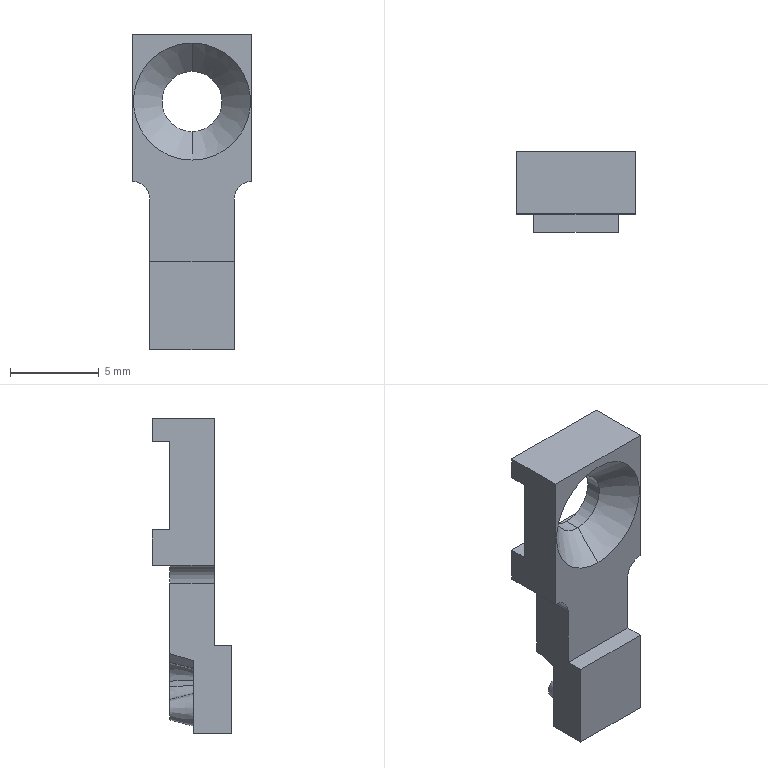Part | SolidWorks | features Cut 6, Chamfer 2, ICE 2, Extrusion 1, Fillet 1, HoleWzd 1 | 1 solid | 35 faces | box 6.75 x 4.5 x 17.8 mm | volume 246.564 mm3 | plane 23 | cone 8 | cylinder 4 | commonest cylinder face diameters 2 x2 3.4 x2
STEP:
#1=CARTESIAN_POINT('',(0.,-1.9,7.15));
#2=VERTEX_POINT('',#1);
#3=CARTESIAN_POINT('',(0.,-1.9,3.75));
#4=VERTEX_POINT('',#3);
#5=CARTESIAN_POINT('',(0.,-1.9,5.45));
#6=DIRECTION('',(0.,-1.,0.));
#7=DIRECTION('',(0.,0.,-1.));
#8=AXIS2_PLACEMENT_3D('',#5,#6,#7);
#9=CIRCLE('',#8,1.7);
#10=EDGE_CURVE('',#2,#4,#9,.T.);
#11=ORIENTED_EDGE('',*,*,#10,.F.);
#12=CARTESIAN_POINT('',(0.,-3.5,8.75));
#13=VERTEX_POINT('',#12);
#14=CARTESIAN_POINT('',(0.,-3.5,8.75));
#15=DIRECTION('',(0.,-0.7071,0.7071));
#16=VECTOR('',#15,1000.);
#17=LINE('',#14,#16);
#18=EDGE_CURVE('',#2,#13,#17,.T.);
#19=ORIENTED_EDGE('',*,*,#18,.T.);
#20=CARTESIAN_POINT('',(0.,-3.5,2.15));
#21=VERTEX_POINT('',#20);
#22=CARTESIAN_POINT('',(0.,-3.5,5.45));
#23=DIRECTION('',(0.,-1.,0.));
#24=DIRECTION('',(0.,0.,-1.));
#25=AXIS2_PLACEMENT_3D('',#22,#23,#24);
#26=CIRCLE('',#25,3.3);
#27=EDGE_CURVE('',#13,#21,#26,.T.);
#28=ORIENTED_EDGE('',*,*,#27,.T.);
#29=CARTESIAN_POINT('',(0.,-3.5,2.15));
#30=DIRECTION('',(0.,-0.7071,-0.7071));
#31=VECTOR('',#30,1000.);
#32=LINE('',#29,#31);
#33=EDGE_CURVE('',#4,#21,#32,.T.);
#34=ORIENTED_EDGE('',*,*,#33,.F.);
#35=EDGE_LOOP('',(#11,#19,#28,#34));
#36=FACE_OUTER_BOUND('',#35,.T.);
#37=CARTESIAN_POINT('',(0.,-3.5,5.45));
#38=DIRECTION('',(0.,-1.,0.));
#39=DIRECTION('',(0.,0.,-1.));
#40=AXIS2_PLACEMENT_3D('',#37,#38,#39);
#41=CONICAL_SURFACE('',#40,3.3,0.7854);
#42=ADVANCED_FACE('',(#36),#41,.F.);
#43=CARTESIAN_POINT('',(0.,-1.,7.15));
#44=VERTEX_POINT('',#43);
#45=CARTESIAN_POINT('',(0.,-1.,3.75));
#46=VERTEX_POINT('',#45);
#47=CARTESIAN_POINT('',(0.,-1.,5.45));
#48=DIRECTION('',(0.,-1.,0.));
#49=DIRECTION('',(0.,0.,-1.));
#50=AXIS2_PLACEMENT_3D('',#47,#48,#49);
#51=CIRCLE('',#50,1.7);
#52=EDGE_CURVE('',#44,#46,#51,.T.);
#53=ORIENTED_EDGE('',*,*,#52,.F.);
#54=CARTESIAN_POINT('',(0.,-3.5,7.15));
#55=DIRECTION('',(0.,-1.,0.));
#56=VECTOR('',#55,1000.);
#57=LINE('',#54,#56);
#58=EDGE_CURVE('',#44,#2,#57,.T.);
#59=ORIENTED_EDGE('',*,*,#58,.T.);
#60=ORIENTED_EDGE('',*,*,#10,.T.);
#61=CARTESIAN_POINT('',(0.,-3.5,3.75));
#62=DIRECTION('',(0.,-1.,0.));
#63=VECTOR('',#62,1000.);
#64=LINE('',#61,#63);
#65=EDGE_CURVE('',#46,#4,#64,.T.);
#66=ORIENTED_EDGE('',*,*,#65,.F.);
#67=EDGE_LOOP('',(#53,#59,#60,#66));
#68=FACE_OUTER_BOUND('',#67,.T.);
#69=CARTESIAN_POINT('',(0.,-3.5,5.45));
#70=DIRECTION('',(0.,-1.,0.));
#71=DIRECTION('',(0.,0.,-1.));
#72=AXIS2_PLACEMENT_3D('',#69,#70,#71);
#73=CYLINDRICAL_SURFACE('',#72,1.7);
#74=ADVANCED_FACE('',(#68),#73,.F.);
#75=CARTESIAN_POINT('',(-1.503,-1.,-4.523));
#76=VERTEX_POINT('',#75);
#77=CARTESIAN_POINT('',(-1.512,-1.,-4.52));
#78=VERTEX_POINT('',#77);
#79=CARTESIAN_POINT('',(-1.503,-1.,-4.505));
#80=DIRECTION('',(0.,1.,0.));
#81=DIRECTION('',(0.,0.,-1.));
#82=AXIS2_PLACEMENT_3D('',#79,#80,#81);
#83=CIRCLE('',#82,0.01769);
#84=EDGE_CURVE('',#76,#78,#83,.T.);
#85=ORIENTED_EDGE('',*,*,#84,.T.);
#86=CARTESIAN_POINT('',(-2.375,-1.,-4.022));
#87=VERTEX_POINT('',#86);
#88=CARTESIAN_POINT('',(-5.278,-1.,-2.346));
#89=DIRECTION('',(-0.866,0.,0.5));
#90=VECTOR('',#89,1000.);
#91=LINE('',#88,#90);
#92=EDGE_CURVE('',#78,#87,#91,.T.);
#93=ORIENTED_EDGE('',*,*,#92,.T.);
#94=CARTESIAN_POINT('',(-2.375,-1.,-0.05));
#95=VERTEX_POINT('',#94);
#96=CARTESIAN_POINT('',(-2.375,-1.,-0.05));
#97=DIRECTION('',(0.,0.,1.));
#98=VECTOR('',#97,1000.);
#99=LINE('',#96,#98);
#100=EDGE_CURVE('',#87,#95,#99,.T.);
#101=ORIENTED_EDGE('',*,*,#100,.T.);
#102=CARTESIAN_POINT('',(-3.375,-1.,0.95));
#103=VERTEX_POINT('',#102);
#104=CARTESIAN_POINT('',(-3.375,-1.,-0.05));
#105=DIRECTION('',(0.,-1.,0.));
#106=DIRECTION('',(0.,0.,-1.));
#107=AXIS2_PLACEMENT_3D('',#104,#105,#106);
#108=CIRCLE('',#107,1.);
#109=EDGE_CURVE('',#95,#103,#108,.T.);
#110=ORIENTED_EDGE('',*,*,#109,.T.);
#111=CARTESIAN_POINT('',(3.375,-1.,0.95));
#112=VERTEX_POINT('',#111);
#113=CARTESIAN_POINT('',(-3.375,-1.,0.95));
#114=DIRECTION('',(1.,0.,0.));
#115=VECTOR('',#114,1000.);
#116=LINE('',#113,#115);
#117=EDGE_CURVE('',#103,#112,#116,.T.);
#118=ORIENTED_EDGE('',*,*,#117,.T.);
#119=CARTESIAN_POINT('',(2.375,-1.,-0.05));
#120=VERTEX_POINT('',#119);
#121=CARTESIAN_POINT('',(3.375,-1.,-0.05));
#122=DIRECTION('',(0.,-1.,0.));
#123=DIRECTION('',(0.,0.,-1.));
#124=AXIS2_PLACEMENT_3D('',#121,#122,#123);
#125=CIRCLE('',#124,1.);
#126=EDGE_CURVE('',#112,#120,#125,.T.);
#127=ORIENTED_EDGE('',*,*,#126,.T.);
#128=CARTESIAN_POINT('',(2.375,-1.,-7.053));
#129=VERTEX_POINT('',#128);
#130=CARTESIAN_POINT('',(2.375,-1.,-0.05));
#131=DIRECTION('',(0.,0.,-1.));
#132=VECTOR('',#131,1000.);
#133=LINE('',#130,#132);
#134=EDGE_CURVE('',#120,#129,#133,.T.);
#135=ORIENTED_EDGE('',*,*,#134,.T.);
#136=CARTESIAN_POINT('',(2.276,-1.,-7.225));
#137=VERTEX_POINT('',#136);
#138=CARTESIAN_POINT('',(4.403,-1.,-3.54));
#139=DIRECTION('',(-0.5,0.,-0.866));
#140=VECTOR('',#139,1000.);
#141=LINE('',#138,#140);
#142=EDGE_CURVE('',#129,#137,#141,.T.);
#143=ORIENTED_EDGE('',*,*,#142,.T.);
#144=CARTESIAN_POINT('',(0.8678,-1.,-7.225));
#145=VERTEX_POINT('',#144);
#146=CARTESIAN_POINT('',(-3.375,-1.,-7.225));
#147=DIRECTION('',(-1.,0.,0.));
#148=VECTOR('',#147,1000.);
#149=LINE('',#146,#148);
#150=EDGE_CURVE('',#137,#145,#149,.T.);
#151=ORIENTED_EDGE('',*,*,#150,.T.);
#152=CARTESIAN_POINT('',(0.8626,-1.,-7.224));
#153=VERTEX_POINT('',#152);
#154=CARTESIAN_POINT('',(0.8678,-1.,-7.207));
#155=DIRECTION('',(0.,1.,0.));
#156=DIRECTION('',(0.,0.,-1.));
#157=AXIS2_PLACEMENT_3D('',#154,#155,#156);
#158=CIRCLE('',#157,0.01769);
#159=EDGE_CURVE('',#145,#153,#158,.T.);
#160=ORIENTED_EDGE('',*,*,#159,.T.);
#161=CARTESIAN_POINT('',(0.6636,-1.,-7.163));
#162=VERTEX_POINT('',#161);
#163=CARTESIAN_POINT('',(-5.298,-1.,-5.34));
#164=DIRECTION('',(-0.9563,0.,0.2924));
#165=VECTOR('',#164,1000.);
#166=LINE('',#163,#165);
#167=EDGE_CURVE('',#153,#162,#166,.T.);
#168=ORIENTED_EDGE('',*,*,#167,.T.);
#169=CARTESIAN_POINT('',(-0.4201,-1.,-7.527));
#170=VERTEX_POINT('',#169);
#171=CARTESIAN_POINT('',(0.3764,-1.,-8.102));
#172=DIRECTION('',(0.,-1.,0.));
#173=DIRECTION('',(0.,0.,-1.));
#174=AXIS2_PLACEMENT_3D('',#171,#172,#173);
#175=CIRCLE('',#174,0.9823);
#176=EDGE_CURVE('',#162,#170,#175,.T.);
#177=ORIENTED_EDGE('',*,*,#176,.T.);
#178=CARTESIAN_POINT('',(-0.9183,-1.,-6.629));
#179=VERTEX_POINT('',#178);
#180=CARTESIAN_POINT('',(-0.8804,-1.,-7.195));
#181=DIRECTION('',(0.,1.,0.));
#182=DIRECTION('',(0.,0.,-1.));
#183=AXIS2_PLACEMENT_3D('',#180,#181,#182);
#184=CIRCLE('',#183,0.5677);
#185=EDGE_CURVE('',#170,#179,#184,.T.);
#186=ORIENTED_EDGE('',*,*,#185,.T.);
#187=CARTESIAN_POINT('',(-0.03484,-1.,-5.903));
#188=VERTEX_POINT('',#187);
#189=CARTESIAN_POINT('',(-0.9837,-1.,-5.649));
#190=DIRECTION('',(0.,-1.,0.));
#191=DIRECTION('',(0.,0.,-1.));
#192=AXIS2_PLACEMENT_3D('',#189,#190,#191);
#193=CIRCLE('',#192,0.9823);
#194=EDGE_CURVE('',#179,#188,#193,.T.);
#195=ORIENTED_EDGE('',*,*,#194,.T.);
#196=CARTESIAN_POINT('',(0.05202,-1.,-5.579));
#197=VERTEX_POINT('',#196);
#198=CARTESIAN_POINT('',(1.455,-1.,-0.3441));
#199=DIRECTION('',(0.2588,0.,0.9659));
#200=VECTOR('',#199,1000.);
#201=LINE('',#198,#200);
#202=EDGE_CURVE('',#188,#197,#201,.T.);
#203=ORIENTED_EDGE('',*,*,#202,.T.);
#204=CARTESIAN_POINT('',(-0.9275,-1.,-4.523));
#205=VERTEX_POINT('',#204);
#206=CARTESIAN_POINT('',(-0.9275,-1.,-5.505));
#207=DIRECTION('',(0.,-1.,0.));
#208=DIRECTION('',(0.,0.,-1.));
#209=AXIS2_PLACEMENT_3D('',#206,#207,#208);
#210=CIRCLE('',#209,0.9823);
#211=EDGE_CURVE('',#197,#205,#210,.T.);
#212=ORIENTED_EDGE('',*,*,#211,.T.);
#213=CARTESIAN_POINT('',(-3.375,-1.,-4.523));
#214=DIRECTION('',(-1.,0.,0.));
#215=VECTOR('',#214,1000.);
#216=LINE('',#213,#215);
#217=EDGE_CURVE('',#205,#76,#216,.T.);
#218=ORIENTED_EDGE('',*,*,#217,.T.);
#219=EDGE_LOOP('',(#85,#93,#101,#110,#118,#127,#135,#143,#151,#160,#168,#177,#186,#195,#203,#212,#218));
#220=FACE_OUTER_BOUND('',#219,.T.);
#221=CARTESIAN_POINT('',(-3.375,-1.,0.95));
#222=DIRECTION('',(0.,-1.,0.));
#223=DIRECTION('',(0.,0.,-1.));
#224=AXIS2_PLACEMENT_3D('',#221,#222,#223);
#225=PLANE('',#224);
#226=ADVANCED_FACE('',(#220),#225,.F.);
#227=CARTESIAN_POINT('',(0.,-3.5,5.45));
#228=DIRECTION('',(0.,-1.,0.));
#229=DIRECTION('',(0.,0.,-1.));
#230=AXIS2_PLACEMENT_3D('',#227,#228,#229);
#231=CIRCLE('',#230,3.3);
#232=EDGE_CURVE('',#21,#13,#231,.T.);
#233=ORIENTED_EDGE('',*,*,#232,.F.);
#234=ORIENTED_EDGE('',*,*,#27,.F.);
#235=EDGE_LOOP('',(#233,#234));
#236=FACE_BOUND('',#235,.T.);
#237=CARTESIAN_POINT('',(2.375,-3.5,-3.55));
#238=VERTEX_POINT('',#237);
#239=CARTESIAN_POINT('',(-2.375,-3.5,-3.55));
#240=VERTEX_POINT('',#239);
#241=CARTESIAN_POINT('',(2.375,-3.5,-3.55));
#242=DIRECTION('',(-1.,0.,0.));
#243=VECTOR('',#242,1000.);
#244=LINE('',#241,#243);
#245=EDGE_CURVE('',#238,#240,#244,.T.);
#246=ORIENTED_EDGE('',*,*,#245,.F.);
#247=CARTESIAN_POINT('',(2.375,-3.5,-0.05));
#248=VERTEX_POINT('',#247);
#249=CARTESIAN_POINT('',(2.375,-3.5,-0.05));
#250=DIRECTION('',(0.,0.,1.));
#251=VECTOR('',#250,1000.);
#252=LINE('',#249,#251);
#253=EDGE_CURVE('',#238,#248,#252,.T.);
#254=ORIENTED_EDGE('',*,*,#253,.T.);
#255=CARTESIAN_POINT('',(3.375,-3.5,0.95));
#256=VERTEX_POINT('',#255);
#257=CARTESIAN_POINT('',(3.375,-3.5,-0.05));
#258=DIRECTION('',(0.,1.,0.));
#259=DIRECTION('',(0.,0.,1.));
#260=AXIS2_PLACEMENT_3D('',#257,#258,#259);
#261=CIRCLE('',#260,1.);
#262=EDGE_CURVE('',#248,#256,#261,.T.);
#263=ORIENTED_EDGE('',*,*,#262,.T.);
#264=CARTESIAN_POINT('',(3.375,-3.5,9.25));
#265=VERTEX_POINT('',#264);
#266=CARTESIAN_POINT('',(3.375,-3.5,9.25));
#267=DIRECTION('',(0.,0.,1.));
#268=VECTOR('',#267,1000.);
#269=LINE('',#266,#268);
#270=EDGE_CURVE('',#256,#265,#269,.T.);
#271=ORIENTED_EDGE('',*,*,#270,.T.);
#272=CARTESIAN_POINT('',(-3.375,-3.5,9.25));
#273=VERTEX_POINT('',#272);
#274=CARTESIAN_POINT('',(-3.375,-3.5,9.25));
#275=DIRECTION('',(1.,0.,0.));
#276=VECTOR('',#275,1000.);
#277=LINE('',#274,#276);
#278=EDGE_CURVE('',#273,#265,#277,.T.);
#279=ORIENTED_EDGE('',*,*,#278,.F.);
#280=CARTESIAN_POINT('',(-3.375,-3.5,0.95));
#281=VERTEX_POINT('',#280);
#282=CARTESIAN_POINT('',(-3.375,-3.5,9.25));
#283=DIRECTION('',(0.,0.,1.));
#284=VECTOR('',#283,1000.);
#285=LINE('',#282,#284);
#286=EDGE_CURVE('',#281,#273,#285,.T.);
#287=ORIENTED_EDGE('',*,*,#286,.F.);
#288=CARTESIAN_POINT('',(-2.375,-3.5,-0.05));
#289=VERTEX_POINT('',#288);
#290=CARTESIAN_POINT('',(-3.375,-3.5,-0.05));
#291=DIRECTION('',(0.,1.,0.));
#292=DIRECTION('',(0.,0.,1.));
#293=AXIS2_PLACEMENT_3D('',#290,#291,#292);
#294=CIRCLE('',#293,1.);
#295=EDGE_CURVE('',#281,#289,#294,.T.);
#296=ORIENTED_EDGE('',*,*,#295,.T.);
#297=CARTESIAN_POINT('',(-2.375,-3.5,-0.05));
#298=DIRECTION('',(0.,0.,-1.));
#299=VECTOR('',#298,1000.);
#300=LINE('',#297,#299);
#301=EDGE_CURVE('',#289,#240,#300,.T.);
#302=ORIENTED_EDGE('',*,*,#301,.T.);
#303=EDGE_LOOP('',(#246,#254,#263,#271,#279,#287,#296,#302));
#304=FACE_OUTER_BOUND('',#303,.T.);
#305=CARTESIAN_POINT('',(-3.375,-3.5,9.25));
#306=DIRECTION('',(0.,1.,0.));
#307=DIRECTION('',(0.,0.,1.));
#308=AXIS2_PLACEMENT_3D('',#305,#306,#307);
#309=PLANE('',#308);
#310=ADVANCED_FACE('',(#236,#304),#309,.F.);
#311=CARTESIAN_POINT('',(3.375,0.,9.25));
#312=VERTEX_POINT('',#311);
#313=CARTESIAN_POINT('',(3.375,0.,7.95));
#314=VERTEX_POINT('',#313);
#315=CARTESIAN_POINT('',(3.375,0.,9.25));
#316=DIRECTION('',(0.,0.,-1.));
#317=VECTOR('',#316,1000.);
#318=LINE('',#315,#317);
#319=EDGE_CURVE('',#312,#314,#318,.T.);
#320=ORIENTED_EDGE('',*,*,#319,.T.);
#321=CARTESIAN_POINT('',(-3.375,0.,7.95));
#322=VERTEX_POINT('',#321);
#323=CARTESIAN_POINT('',(-3.375,0.,7.95));
#324=DIRECTION('',(1.,0.,0.));
#325=VECTOR('',#324,1000.);
#326=LINE('',#323,#325);
#327=EDGE_CURVE('',#322,#314,#326,.T.);
#328=ORIENTED_EDGE('',*,*,#327,.F.);
#329=CARTESIAN_POINT('',(-3.375,0.,9.25));
#330=VERTEX_POINT('',#329);
#331=CARTESIAN_POINT('',(-3.375,0.,9.25));
#332=DIRECTION('',(0.,0.,1.));
#333=VECTOR('',#332,1000.);
#334=LINE('',#331,#333);
#335=EDGE_CURVE('',#322,#330,#334,.T.);
#336=ORIENTED_EDGE('',*,*,#335,.T.);
#337=CARTESIAN_POINT('',(-3.375,0.,9.25));
#338=DIRECTION('',(1.,0.,0.));
#339=VECTOR('',#338,1000.);
#340=LINE('',#337,#339);
#341=EDGE_CURVE('',#330,#312,#340,.T.);
#342=ORIENTED_EDGE('',*,*,#341,.T.);
#343=EDGE_LOOP('',(#320,#328,#336,#342));
#344=FACE_OUTER_BOUND('',#343,.T.);
#345=CARTESIAN_POINT('',(0.,0.,0.));
#346=DIRECTION('',(0.,-1.,0.));
#347=DIRECTION('',(0.,0.,-1.));
#348=AXIS2_PLACEMENT_3D('',#345,#346,#347);
#349=PLANE('',#348);
#350=ADVANCED_FACE('',(#344),#349,.F.);
#351=ORIENTED_EDGE('',*,*,#270,.F.);
#352=CARTESIAN_POINT('',(3.375,0.,0.95));
#353=DIRECTION('',(0.,-1.,0.));
#354=VECTOR('',#353,1000.);
#355=LINE('',#352,#354);
#356=EDGE_CURVE('',#112,#256,#355,.T.);
#357=ORIENTED_EDGE('',*,*,#356,.F.);
#358=CARTESIAN_POINT('',(3.375,0.,0.95));
#359=VERTEX_POINT('',#358);
#360=CARTESIAN_POINT('',(3.375,0.,0.95));
#361=DIRECTION('',(0.,-1.,0.));
#362=VECTOR('',#361,1000.);
#363=LINE('',#360,#362);
#364=EDGE_CURVE('',#359,#112,#363,.T.);
#365=ORIENTED_EDGE('',*,*,#364,.F.);
#366=CARTESIAN_POINT('',(3.375,0.,2.95));
#367=VERTEX_POINT('',#366);
#368=CARTESIAN_POINT('',(3.375,0.,9.25));
#369=DIRECTION('',(0.,0.,-1.));
#370=VECTOR('',#369,1000.);
#371=LINE('',#368,#370);
#372=EDGE_CURVE('',#367,#359,#371,.T.);
#373=ORIENTED_EDGE('',*,*,#372,.F.);
#374=CARTESIAN_POINT('',(3.375,-1.,2.95));
#375=VERTEX_POINT('',#374);
#376=CARTESIAN_POINT('',(3.375,0.,2.95));
#377=DIRECTION('',(0.,1.,0.));
#378=VECTOR('',#377,1000.);
#379=LINE('',#376,#378);
#380=EDGE_CURVE('',#375,#367,#379,.T.);
#381=ORIENTED_EDGE('',*,*,#380,.F.);
#382=CARTESIAN_POINT('',(3.375,-1.,7.95));
#383=VERTEX_POINT('',#382);
#384=CARTESIAN_POINT('',(3.375,-1.,7.95));
#385=DIRECTION('',(0.,0.,-1.));
#386=VECTOR('',#385,1000.);
#387=LINE('',#384,#386);
#388=EDGE_CURVE('',#383,#375,#387,.T.);
#389=ORIENTED_EDGE('',*,*,#388,.F.);
#390=CARTESIAN_POINT('',(3.375,0.,7.95));
#391=DIRECTION('',(0.,-1.,0.));
#392=VECTOR('',#391,1000.);
#393=LINE('',#390,#392);
#394=EDGE_CURVE('',#314,#383,#393,.T.);
#395=ORIENTED_EDGE('',*,*,#394,.F.);
#396=ORIENTED_EDGE('',*,*,#319,.F.);
#397=CARTESIAN_POINT('',(3.375,-5.2,9.25));
#398=DIRECTION('',(0.,1.,0.));
#399=VECTOR('',#398,1000.);
#400=LINE('',#397,#399);
#401=EDGE_CURVE('',#265,#312,#400,.T.);
#402=ORIENTED_EDGE('',*,*,#401,.F.);
#403=EDGE_LOOP('',(#351,#357,#365,#373,#381,#389,#395,#396,#402));
#404=FACE_OUTER_BOUND('',#403,.T.);
#405=CARTESIAN_POINT('',(3.375,-5.2,9.25));
#406=DIRECTION('',(1.,0.,0.));
#407=DIRECTION('',(0.,0.,-1.));
#408=AXIS2_PLACEMENT_3D('',#405,#406,#407);
#409=PLANE('',#408);
#410=ADVANCED_FACE('',(#404),#409,.T.);
#411=ORIENTED_EDGE('',*,*,#278,.T.);
#412=ORIENTED_EDGE('',*,*,#401,.T.);
#413=ORIENTED_EDGE('',*,*,#341,.F.);
#414=CARTESIAN_POINT('',(-3.375,-5.2,9.25));
#415=DIRECTION('',(0.,1.,0.));
#416=VECTOR('',#415,1000.);
#417=LINE('',#414,#416);
#418=EDGE_CURVE('',#273,#330,#417,.T.);
#419=ORIENTED_EDGE('',*,*,#418,.F.);
#420=EDGE_LOOP('',(#411,#412,#413,#419));
#421=FACE_OUTER_BOUND('',#420,.T.);
#422=CARTESIAN_POINT('',(-3.375,-5.2,9.25));
#423=DIRECTION('',(0.,0.,1.));
#424=DIRECTION('',(1.,0.,0.));
#425=AXIS2_PLACEMENT_3D('',#422,#423,#424);
#426=PLANE('',#425);
#427=ADVANCED_FACE('',(#421),#426,.T.);
#428=CARTESIAN_POINT('',(-3.375,0.,0.95));
#429=VERTEX_POINT('',#428);
#430=CARTESIAN_POINT('',(-3.375,0.,0.95));
#431=DIRECTION('',(0.,-1.,0.));
#432=VECTOR('',#431,1000.);
#433=LINE('',#430,#432);
#434=EDGE_CURVE('',#429,#103,#433,.T.);
#435=ORIENTED_EDGE('',*,*,#434,.T.);
#436=CARTESIAN_POINT('',(-3.375,0.,0.95));
#437=DIRECTION('',(0.,-1.,0.));
#438=VECTOR('',#437,1000.);
#439=LINE('',#436,#438);
#440=EDGE_CURVE('',#103,#281,#439,.T.);
#441=ORIENTED_EDGE('',*,*,#440,.T.);
#442=ORIENTED_EDGE('',*,*,#286,.T.);
#443=ORIENTED_EDGE('',*,*,#418,.T.);
#444=ORIENTED_EDGE('',*,*,#335,.F.);
#445=CARTESIAN_POINT('',(-3.375,-1.,7.95));
#446=VERTEX_POINT('',#445);
#447=CARTESIAN_POINT('',(-3.375,0.,7.95));
#448=DIRECTION('',(0.,-1.,0.));
#449=VECTOR('',#448,1000.);
#450=LINE('',#447,#449);
#451=EDGE_CURVE('',#322,#446,#450,.T.);
#452=ORIENTED_EDGE('',*,*,#451,.T.);
#453=CARTESIAN_POINT('',(-3.375,-1.,2.95));
#454=VERTEX_POINT('',#453);
#455=CARTESIAN_POINT('',(-3.375,-1.,7.95));
#456=DIRECTION('',(0.,0.,-1.));
#457=VECTOR('',#456,1000.);
#458=LINE('',#455,#457);
#459=EDGE_CURVE('',#446,#454,#458,.T.);
#460=ORIENTED_EDGE('',*,*,#459,.T.);
#461=CARTESIAN_POINT('',(-3.375,0.,2.95));
#462=VERTEX_POINT('',#461);
#463=CARTESIAN_POINT('',(-3.375,0.,2.95));
#464=DIRECTION('',(0.,1.,0.));
#465=VECTOR('',#464,1000.);
#466=LINE('',#463,#465);
#467=EDGE_CURVE('',#454,#462,#466,.T.);
#468=ORIENTED_EDGE('',*,*,#467,.T.);
#469=CARTESIAN_POINT('',(-3.375,0.,9.25));
#470=DIRECTION('',(0.,0.,1.));
#471=VECTOR('',#470,1000.);
#472=LINE('',#469,#471);
#473=EDGE_CURVE('',#429,#462,#472,.T.);
#474=ORIENTED_EDGE('',*,*,#473,.F.);
#475=EDGE_LOOP('',(#435,#441,#442,#443,#444,#452,#460,#468,#474));
#476=FACE_OUTER_BOUND('',#475,.T.);
#477=CARTESIAN_POINT('',(-3.375,-5.2,9.25));
#478=DIRECTION('',(-1.,0.,0.));
#479=DIRECTION('',(0.,0.,1.));
#480=AXIS2_PLACEMENT_3D('',#477,#478,#479);
#481=PLANE('',#480);
#482=ADVANCED_FACE('',(#476),#481,.T.);
#483=ORIENTED_EDGE('',*,*,#372,.T.);
#484=CARTESIAN_POINT('',(-3.375,0.,0.95));
#485=DIRECTION('',(1.,0.,0.));
#486=VECTOR('',#485,1000.);
#487=LINE('',#484,#486);
#488=EDGE_CURVE('',#429,#359,#487,.T.);
#489=ORIENTED_EDGE('',*,*,#488,.F.);
#490=ORIENTED_EDGE('',*,*,#473,.T.);
#491=CARTESIAN_POINT('',(-3.375,0.,2.95));
#492=DIRECTION('',(1.,0.,0.));
#493=VECTOR('',#492,1000.);
#494=LINE('',#491,#493);
#495=EDGE_CURVE('',#462,#367,#494,.T.);
#496=ORIENTED_EDGE('',*,*,#495,.T.);
#497=EDGE_LOOP('',(#483,#489,#490,#496));
#498=FACE_OUTER_BOUND('',#497,.T.);
#499=CARTESIAN_POINT('',(0.,0.,0.));
#500=DIRECTION('',(0.,-1.,0.));
#501=DIRECTION('',(0.,0.,-1.));
#502=AXIS2_PLACEMENT_3D('',#499,#500,#501);
#503=PLANE('',#502);
#504=ADVANCED_FACE('',(#498),#503,.F.);
#505=ORIENTED_EDGE('',*,*,#394,.T.);
#506=CARTESIAN_POINT('',(-3.375,-1.,7.95));
#507=DIRECTION('',(1.,0.,0.));
#508=VECTOR('',#507,1000.);
#509=LINE('',#506,#508);
#510=EDGE_CURVE('',#446,#383,#509,.T.);
#511=ORIENTED_EDGE('',*,*,#510,.F.);
#512=ORIENTED_EDGE('',*,*,#451,.F.);
#513=ORIENTED_EDGE('',*,*,#327,.T.);
#514=EDGE_LOOP('',(#505,#511,#512,#513));
#515=FACE_OUTER_BOUND('',#514,.T.);
#516=CARTESIAN_POINT('',(-3.375,0.,7.95));
#517=DIRECTION('',(0.,0.,1.));
#518=DIRECTION('',(1.,0.,0.));
#519=AXIS2_PLACEMENT_3D('',#516,#517,#518);
#520=PLANE('',#519);
#521=ADVANCED_FACE('',(#515),#520,.F.);
#522=ORIENTED_EDGE('',*,*,#380,.T.);
#523=ORIENTED_EDGE('',*,*,#495,.F.);
#524=ORIENTED_EDGE('',*,*,#467,.F.);
#525=CARTESIAN_POINT('',(-3.375,-1.,2.95));
#526=DIRECTION('',(1.,0.,0.));
#527=VECTOR('',#526,1000.);
#528=LINE('',#525,#527);
#529=EDGE_CURVE('',#454,#375,#528,.T.);
#530=ORIENTED_EDGE('',*,*,#529,.T.);
#531=EDGE_LOOP('',(#522,#523,#524,#530));
#532=FACE_OUTER_BOUND('',#531,.T.);
#533=CARTESIAN_POINT('',(-3.375,0.,2.95));
#534=DIRECTION('',(0.,0.,-1.));
#535=DIRECTION('',(-1.,0.,0.));
#536=AXIS2_PLACEMENT_3D('',#533,#534,#535);
#537=PLANE('',#536);
#538=ADVANCED_FACE('',(#532),#537,.F.);
#539=CARTESIAN_POINT('',(0.,-1.,5.45));
#540=DIRECTION('',(0.,-1.,0.));
#541=DIRECTION('',(0.,0.,-1.));
#542=AXIS2_PLACEMENT_3D('',#539,#540,#541);
#543=CIRCLE('',#542,1.7);
#544=EDGE_CURVE('',#46,#44,#543,.T.);
#545=ORIENTED_EDGE('',*,*,#544,.T.);
#546=ORIENTED_EDGE('',*,*,#52,.T.);
#547=EDGE_LOOP('',(#545,#546));
#548=FACE_BOUND('',#547,.T.);
#549=ORIENTED_EDGE('',*,*,#388,.T.);
#550=ORIENTED_EDGE('',*,*,#529,.F.);
#551=ORIENTED_EDGE('',*,*,#459,.F.);
#552=ORIENTED_EDGE('',*,*,#510,.T.);
#553=EDGE_LOOP('',(#549,#550,#551,#552));
#554=FACE_OUTER_BOUND('',#553,.T.);
#555=CARTESIAN_POINT('',(-3.375,-1.,7.95));
#556=DIRECTION('',(0.,-1.,0.));
#557=DIRECTION('',(0.,0.,-1.));
#558=AXIS2_PLACEMENT_3D('',#555,#556,#557);
#559=PLANE('',#558);
#560=ADVANCED_FACE('',(#548,#554),#559,.F.);
#561=ORIENTED_EDGE('',*,*,#364,.T.);
#562=ORIENTED_EDGE('',*,*,#117,.F.);
#563=ORIENTED_EDGE('',*,*,#434,.F.);
#564=ORIENTED_EDGE('',*,*,#488,.T.);
#565=EDGE_LOOP('',(#561,#562,#563,#564));
#566=FACE_OUTER_BOUND('',#565,.T.);
#567=CARTESIAN_POINT('',(-3.375,0.,0.95));
#568=DIRECTION('',(0.,0.,1.));
#569=DIRECTION('',(0.,-1.,0.));
#570=AXIS2_PLACEMENT_3D('',#567,#568,#569);
#571=PLANE('',#570);
#572=ADVANCED_FACE('',(#566),#571,.F.);
#573=ORIENTED_EDGE('',*,*,#58,.F.);
#574=ORIENTED_EDGE('',*,*,#544,.F.);
#575=ORIENTED_EDGE('',*,*,#65,.T.);
#576=CARTESIAN_POINT('',(0.,-1.9,5.45));
#577=DIRECTION('',(0.,-1.,0.));
#578=DIRECTION('',(0.,0.,-1.));
#579=AXIS2_PLACEMENT_3D('',#576,#577,#578);
#580=CIRCLE('',#579,1.7);
#581=EDGE_CURVE('',#4,#2,#580,.T.);
#582=ORIENTED_EDGE('',*,*,#581,.T.);
#583=EDGE_LOOP('',(#573,#574,#575,#582));
#584=FACE_OUTER_BOUND('',#583,.T.);
#585=CARTESIAN_POINT('',(0.,-3.5,5.45));
#586=DIRECTION('',(0.,-1.,0.));
#587=DIRECTION('',(0.,0.,-1.));
#588=AXIS2_PLACEMENT_3D('',#585,#586,#587);
#589=CYLINDRICAL_SURFACE('',#588,1.7);
#590=ADVANCED_FACE('',(#584),#589,.F.);
#591=ORIENTED_EDGE('',*,*,#18,.F.);
#592=ORIENTED_EDGE('',*,*,#581,.F.);
#593=ORIENTED_EDGE('',*,*,#33,.T.);
#594=ORIENTED_EDGE('',*,*,#232,.T.);
#595=EDGE_LOOP('',(#591,#592,#593,#594));
#596=FACE_OUTER_BOUND('',#595,.T.);
#597=CARTESIAN_POINT('',(0.,-3.5,5.45));
#598=DIRECTION('',(0.,-1.,0.));
#599=DIRECTION('',(0.,0.,-1.));
#600=AXIS2_PLACEMENT_3D('',#597,#598,#599);
#601=CONICAL_SURFACE('',#600,3.3,0.7854);
#602=ADVANCED_FACE('',(#596),#601,.F.);
#603=ORIENTED_EDGE('',*,*,#262,.F.);
#604=CARTESIAN_POINT('',(2.375,-3.5,-0.05));
#605=DIRECTION('',(0.,-1.,0.));
#606=VECTOR('',#605,1000.);
#607=LINE('',#604,#606);
#608=EDGE_CURVE('',#120,#248,#607,.T.);
#609=ORIENTED_EDGE('',*,*,#608,.F.);
#610=ORIENTED_EDGE('',*,*,#126,.F.);
#611=ORIENTED_EDGE('',*,*,#356,.T.);
#612=EDGE_LOOP('',(#603,#609,#610,#611));
#613=FACE_OUTER_BOUND('',#612,.T.);
#614=CARTESIAN_POINT('',(3.375,0.,-0.05));
#615=DIRECTION('',(0.,-1.,0.));
#616=DIRECTION('',(0.,0.,-1.));
#617=AXIS2_PLACEMENT_3D('',#614,#615,#616);
#618=CYLINDRICAL_SURFACE('',#617,1.);
#619=ADVANCED_FACE('',(#613),#618,.F.);
#620=ORIENTED_EDGE('',*,*,#295,.F.);
#621=ORIENTED_EDGE('',*,*,#440,.F.);
#622=ORIENTED_EDGE('',*,*,#109,.F.);
#623=CARTESIAN_POINT('',(-2.375,-1.,-0.05));
#624=DIRECTION('',(0.,1.,0.));
#625=VECTOR('',#624,1000.);
#626=LINE('',#623,#625);
#627=EDGE_CURVE('',#289,#95,#626,.T.);
#628=ORIENTED_EDGE('',*,*,#627,.F.);
#629=EDGE_LOOP('',(#620,#621,#622,#628));
#630=FACE_OUTER_BOUND('',#629,.T.);
#631=CARTESIAN_POINT('',(-3.375,-5.2,-0.05));
#632=DIRECTION('',(0.,-1.,0.));
#633=DIRECTION('',(0.,0.,-1.));
#634=AXIS2_PLACEMENT_3D('',#631,#632,#633);
#635=CYLINDRICAL_SURFACE('',#634,1.);
#636=ADVANCED_FACE('',(#630),#635,.F.);
#637=CARTESIAN_POINT('',(-2.375,-2.325,-4.432));
#638=VERTEX_POINT('',#637);
#639=CARTESIAN_POINT('',(-2.375,-11.047,-7.13));
#640=DIRECTION('',(0.,-0.9553,-0.2956));
#641=VECTOR('',#640,1000.);
#642=LINE('',#639,#641);
#643=EDGE_CURVE('',#87,#638,#642,.T.);
#644=ORIENTED_EDGE('',*,*,#643,.T.);
#645=CARTESIAN_POINT('',(-2.375,-2.325,-8.55));
#646=VERTEX_POINT('',#645);
#647=CARTESIAN_POINT('',(-2.375,-2.325,-0.05));
#648=DIRECTION('',(0.,0.,1.));
#649=VECTOR('',#648,1000.);
#650=LINE('',#647,#649);
#651=EDGE_CURVE('',#646,#638,#650,.T.);
#652=ORIENTED_EDGE('',*,*,#651,.F.);
#653=CARTESIAN_POINT('',(-2.375,-4.5,-8.55));
#654=VERTEX_POINT('',#653);
#655=CARTESIAN_POINT('',(-2.375,-13.237,-8.55));
#656=DIRECTION('',(0.,1.,0.));
#657=VECTOR('',#656,1000.);
#658=LINE('',#655,#657);
#659=EDGE_CURVE('',#654,#646,#658,.T.);
#660=ORIENTED_EDGE('',*,*,#659,.F.);
#661=CARTESIAN_POINT('',(-2.375,-4.5,-3.55));
#662=VERTEX_POINT('',#661);
#663=CARTESIAN_POINT('',(-2.375,-4.5,-8.55));
#664=DIRECTION('',(0.,0.,-1.));
#665=VECTOR('',#664,1000.);
#666=LINE('',#663,#665);
#667=EDGE_CURVE('',#662,#654,#666,.T.);
#668=ORIENTED_EDGE('',*,*,#667,.F.);
#669=CARTESIAN_POINT('',(-2.375,-4.5,-3.55));
#670=DIRECTION('',(0.,1.,0.));
#671=VECTOR('',#670,1000.);
#672=LINE('',#669,#671);
#673=EDGE_CURVE('',#662,#240,#672,.T.);
#674=ORIENTED_EDGE('',*,*,#673,.T.);
#675=ORIENTED_EDGE('',*,*,#301,.F.);
#676=ORIENTED_EDGE('',*,*,#627,.T.);
#677=ORIENTED_EDGE('',*,*,#100,.F.);
#678=EDGE_LOOP('',(#644,#652,#660,#668,#674,#675,#676,#677));
#679=FACE_OUTER_BOUND('',#678,.T.);
#680=CARTESIAN_POINT('',(-2.375,-13.237,-0.05));
#681=DIRECTION('',(-1.,0.,0.));
#682=DIRECTION('',(0.,0.,1.));
#683=AXIS2_PLACEMENT_3D('',#680,#681,#682);
#684=PLANE('',#683);
#685=ADVANCED_FACE('',(#679),#684,.T.);
#686=CARTESIAN_POINT('',(2.375,-2.325,-8.55));
#687=VERTEX_POINT('',#686);
#688=CARTESIAN_POINT('',(-2.375,-2.325,-8.55));
#689=DIRECTION('',(-1.,0.,0.));
#690=VECTOR('',#689,1000.);
#691=LINE('',#688,#690);
#692=EDGE_CURVE('',#687,#646,#691,.T.);
#693=ORIENTED_EDGE('',*,*,#692,.F.);
#694=CARTESIAN_POINT('',(2.375,-4.5,-8.55));
#695=VERTEX_POINT('',#694);
#696=CARTESIAN_POINT('',(2.375,-13.237,-8.55));
#697=DIRECTION('',(0.,1.,0.));
#698=VECTOR('',#697,1000.);
#699=LINE('',#696,#698);
#700=EDGE_CURVE('',#695,#687,#699,.T.);
#701=ORIENTED_EDGE('',*,*,#700,.F.);
#702=CARTESIAN_POINT('',(2.375,-4.5,-8.55));
#703=DIRECTION('',(1.,0.,0.));
#704=VECTOR('',#703,1000.);
#705=LINE('',#702,#704);
#706=EDGE_CURVE('',#654,#695,#705,.T.);
#707=ORIENTED_EDGE('',*,*,#706,.F.);
#708=ORIENTED_EDGE('',*,*,#659,.T.);
#709=EDGE_LOOP('',(#693,#701,#707,#708));
#710=FACE_OUTER_BOUND('',#709,.T.);
#711=CARTESIAN_POINT('',(-2.375,-13.237,-8.55));
#712=DIRECTION('',(0.,0.,-1.));
#713=DIRECTION('',(-1.,0.,0.));
#714=AXIS2_PLACEMENT_3D('',#711,#712,#713);
#715=PLANE('',#714);
#716=ADVANCED_FACE('',(#710),#715,.T.);
#717=CARTESIAN_POINT('',(2.375,-2.325,-7.053));
#718=VERTEX_POINT('',#717);
#719=CARTESIAN_POINT('',(2.375,-13.237,-7.053));
#720=DIRECTION('',(0.,-1.,0.));
#721=VECTOR('',#720,1000.);
#722=LINE('',#719,#721);
#723=EDGE_CURVE('',#129,#718,#722,.T.);
#724=ORIENTED_EDGE('',*,*,#723,.F.);
#725=ORIENTED_EDGE('',*,*,#134,.F.);
#726=ORIENTED_EDGE('',*,*,#608,.T.);
#727=ORIENTED_EDGE('',*,*,#253,.F.);
#728=CARTESIAN_POINT('',(2.375,-4.5,-3.55));
#729=VERTEX_POINT('',#728);
#730=CARTESIAN_POINT('',(2.375,-4.5,-3.55));
#731=DIRECTION('',(0.,1.,0.));
#732=VECTOR('',#731,1000.);
#733=LINE('',#730,#732);
#734=EDGE_CURVE('',#729,#238,#733,.T.);
#735=ORIENTED_EDGE('',*,*,#734,.F.);
#736=CARTESIAN_POINT('',(2.375,-4.5,-8.55));
#737=DIRECTION('',(0.,0.,1.));
#738=VECTOR('',#737,1000.);
#739=LINE('',#736,#738);
#740=EDGE_CURVE('',#695,#729,#739,.T.);
#741=ORIENTED_EDGE('',*,*,#740,.F.);
#742=ORIENTED_EDGE('',*,*,#700,.T.);
#743=CARTESIAN_POINT('',(2.375,-2.325,-0.05));
#744=DIRECTION('',(0.,0.,-1.));
#745=VECTOR('',#744,1000.);
#746=LINE('',#743,#745);
#747=EDGE_CURVE('',#718,#687,#746,.T.);
#748=ORIENTED_EDGE('',*,*,#747,.F.);
#749=EDGE_LOOP('',(#724,#725,#726,#727,#735,#741,#742,#748));
#750=FACE_OUTER_BOUND('',#749,.T.);
#751=CARTESIAN_POINT('',(2.375,-13.237,-0.05));
#752=DIRECTION('',(1.,0.,0.));
#753=DIRECTION('',(0.,0.,-1.));
#754=AXIS2_PLACEMENT_3D('',#751,#752,#753);
#755=PLANE('',#754);
#756=ADVANCED_FACE('',(#750),#755,.T.);
#757=ORIENTED_EDGE('',*,*,#245,.T.);
#758=ORIENTED_EDGE('',*,*,#673,.F.);
#759=CARTESIAN_POINT('',(2.375,-4.5,-3.55));
#760=DIRECTION('',(-1.,0.,0.));
#761=VECTOR('',#760,1000.);
#762=LINE('',#759,#761);
#763=EDGE_CURVE('',#729,#662,#762,.T.);
#764=ORIENTED_EDGE('',*,*,#763,.F.);
#765=ORIENTED_EDGE('',*,*,#734,.T.);
#766=EDGE_LOOP('',(#757,#758,#764,#765));
#767=FACE_OUTER_BOUND('',#766,.T.);
#768=CARTESIAN_POINT('',(2.375,-4.5,-3.55));
#769=DIRECTION('',(0.,0.,-1.));
#770=DIRECTION('',(-1.,0.,0.));
#771=AXIS2_PLACEMENT_3D('',#768,#769,#770);
#772=PLANE('',#771);
#773=ADVANCED_FACE('',(#767),#772,.F.);
#774=ORIENTED_EDGE('',*,*,#740,.T.);
#775=ORIENTED_EDGE('',*,*,#763,.T.);
#776=ORIENTED_EDGE('',*,*,#667,.T.);
#777=ORIENTED_EDGE('',*,*,#706,.T.);
#778=EDGE_LOOP('',(#774,#775,#776,#777));
#779=FACE_OUTER_BOUND('',#778,.T.);
#780=CARTESIAN_POINT('',(0.,-4.5,0.));
#781=DIRECTION('',(0.,-1.,0.));
#782=DIRECTION('',(0.,0.,-1.));
#783=AXIS2_PLACEMENT_3D('',#780,#781,#782);
#784=PLANE('',#783);
#785=ADVANCED_FACE('',(#779),#784,.T.);
#786=CARTESIAN_POINT('',(2.071,-2.325,-7.58));
#787=VERTEX_POINT('',#786);
#788=CARTESIAN_POINT('',(1.997,-2.325,-7.707));
#789=DIRECTION('',(-0.5,0.,-0.866));
#790=VECTOR('',#789,1000.);
#791=LINE('',#788,#790);
#792=EDGE_CURVE('',#718,#787,#791,.T.);
#793=ORIENTED_EDGE('',*,*,#792,.T.);
#794=CARTESIAN_POINT('',(2.152,-1.798,-7.438));
#795=DIRECTION('',(0.1478,0.9553,0.256));
#796=VECTOR('',#795,1000.);
#797=LINE('',#794,#796);
#798=EDGE_CURVE('',#787,#137,#797,.T.);
#799=ORIENTED_EDGE('',*,*,#798,.T.);
#800=ORIENTED_EDGE('',*,*,#142,.F.);
#801=ORIENTED_EDGE('',*,*,#723,.T.);
#802=EDGE_LOOP('',(#793,#799,#800,#801));
#803=FACE_OUTER_BOUND('',#802,.T.);
#804=CARTESIAN_POINT('',(1.997,0.,-7.707));
#805=DIRECTION('',(-0.866,0.,0.5));
#806=DIRECTION('',(0.5,0.,0.866));
#807=AXIS2_PLACEMENT_3D('',#804,#805,#806);
#808=PLANE('',#807);
#809=ADVANCED_FACE('',(#803),#808,.F.);
#810=ORIENTED_EDGE('',*,*,#651,.T.);
#811=CARTESIAN_POINT('',(-1.689,-2.325,-4.828));
#812=VERTEX_POINT('',#811);
#813=CARTESIAN_POINT('',(1.278,-2.325,-6.541));
#814=DIRECTION('',(0.866,0.,-0.5));
#815=VECTOR('',#814,1000.);
#816=LINE('',#813,#815);
#817=EDGE_CURVE('',#638,#812,#816,.T.);
#818=ORIENTED_EDGE('',*,*,#817,.T.);
#819=CARTESIAN_POINT('',(-1.503,-2.325,-4.878));
#820=VERTEX_POINT('',#819);
#821=CARTESIAN_POINT('',(-1.503,-2.325,-4.505));
#822=DIRECTION('',(0.,-1.,0.));
#823=DIRECTION('',(0.,0.,-1.));
#824=AXIS2_PLACEMENT_3D('',#821,#822,#823);
#825=CIRCLE('',#824,0.3728);
#826=EDGE_CURVE('',#812,#820,#825,.T.);
#827=ORIENTED_EDGE('',*,*,#826,.T.);
#828=CARTESIAN_POINT('',(-0.9275,-2.325,-4.878));
#829=VERTEX_POINT('',#828);
#830=CARTESIAN_POINT('',(0.3764,-2.325,-4.878));
#831=DIRECTION('',(1.,0.,0.));
#832=VECTOR('',#831,1000.);
#833=LINE('',#830,#832);
#834=EDGE_CURVE('',#820,#829,#833,.T.);
#835=ORIENTED_EDGE('',*,*,#834,.T.);
#836=CARTESIAN_POINT('',(-0.3005,-2.325,-5.523));
#837=VERTEX_POINT('',#836);
#838=CARTESIAN_POINT('',(-0.9275,-2.325,-5.505));
#839=DIRECTION('',(0.,1.,0.));
#840=DIRECTION('',(0.,0.,-1.));
#841=AXIS2_PLACEMENT_3D('',#838,#839,#840);
#842=CIRCLE('',#841,0.6272);
#843=EDGE_CURVE('',#829,#837,#842,.T.);
#844=ORIENTED_EDGE('',*,*,#843,.T.);
#845=CARTESIAN_POINT('',(-0.3778,-2.325,-5.811));
#846=VERTEX_POINT('',#845);
#847=CARTESIAN_POINT('',(-0.9001,-2.325,-7.76));
#848=DIRECTION('',(-0.2588,0.,-0.9659));
#849=VECTOR('',#848,1000.);
#850=LINE('',#847,#849);
#851=EDGE_CURVE('',#837,#846,#850,.T.);
#852=ORIENTED_EDGE('',*,*,#851,.T.);
#853=CARTESIAN_POINT('',(-0.9419,-2.325,-6.274));
#854=VERTEX_POINT('',#853);
#855=CARTESIAN_POINT('',(-0.9837,-2.325,-5.649));
#856=DIRECTION('',(0.,1.,0.));
#857=DIRECTION('',(0.,0.,-1.));
#858=AXIS2_PLACEMENT_3D('',#855,#856,#857);
#859=CIRCLE('',#858,0.6272);
#860=EDGE_CURVE('',#846,#854,#859,.T.);
#861=ORIENTED_EDGE('',*,*,#860,.T.);
#862=CARTESIAN_POINT('',(-0.1322,-2.325,-7.735));
#863=VERTEX_POINT('',#862);
#864=CARTESIAN_POINT('',(-0.8804,-2.325,-7.195));
#865=DIRECTION('',(0.,-1.,0.));
#866=DIRECTION('',(0.,0.,-1.));
#867=AXIS2_PLACEMENT_3D('',#864,#865,#866);
#868=CIRCLE('',#867,0.9228);
#869=EDGE_CURVE('',#854,#863,#868,.T.);
#870=ORIENTED_EDGE('',*,*,#869,.T.);
#871=CARTESIAN_POINT('',(0.5598,-2.325,-7.503));
#872=VERTEX_POINT('',#871);
#873=CARTESIAN_POINT('',(0.3764,-2.325,-8.102));
#874=DIRECTION('',(0.,1.,0.));
#875=DIRECTION('',(0.,0.,-1.));
#876=AXIS2_PLACEMENT_3D('',#873,#874,#875);
#877=CIRCLE('',#876,0.6272);
#878=EDGE_CURVE('',#863,#872,#877,.T.);
#879=ORIENTED_EDGE('',*,*,#878,.T.);
#880=CARTESIAN_POINT('',(0.7588,-2.325,-7.563));
#881=VERTEX_POINT('',#880);
#882=CARTESIAN_POINT('',(0.5598,-2.325,-7.503));
#883=DIRECTION('',(0.9563,0.,-0.2924));
#884=VECTOR('',#883,1000.);
#885=LINE('',#882,#884);
#886=EDGE_CURVE('',#872,#881,#885,.T.);
#887=ORIENTED_EDGE('',*,*,#886,.T.);
#888=CARTESIAN_POINT('',(0.8678,-2.325,-7.58));
#889=VERTEX_POINT('',#888);
#890=CARTESIAN_POINT('',(0.8678,-2.325,-7.207));
#891=DIRECTION('',(0.,-1.,0.));
#892=DIRECTION('',(0.,0.,-1.));
#893=AXIS2_PLACEMENT_3D('',#890,#891,#892);
#894=CIRCLE('',#893,0.3728);
#895=EDGE_CURVE('',#881,#889,#894,.T.);
#896=ORIENTED_EDGE('',*,*,#895,.T.);
#897=CARTESIAN_POINT('',(0.3764,-2.325,-7.58));
#898=DIRECTION('',(1.,0.,0.));
#899=VECTOR('',#898,1000.);
#900=LINE('',#897,#899);
#901=EDGE_CURVE('',#889,#787,#900,.T.);
#902=ORIENTED_EDGE('',*,*,#901,.T.);
#903=ORIENTED_EDGE('',*,*,#792,.F.);
#904=ORIENTED_EDGE('',*,*,#747,.T.);
#905=ORIENTED_EDGE('',*,*,#692,.T.);
#906=EDGE_LOOP('',(#810,#818,#827,#835,#844,#852,#861,#870,#879,#887,#896,#902,#903,#904,#905));
#907=FACE_OUTER_BOUND('',#906,.T.);
#908=CARTESIAN_POINT('',(0.3764,-2.325,-8.102));
#909=DIRECTION('',(0.,-1.,0.));
#910=DIRECTION('',(0.,0.,-1.));
#911=AXIS2_PLACEMENT_3D('',#908,#909,#910);
#912=PLANE('',#911);
#913=ADVANCED_FACE('',(#907),#912,.F.);
#914=ORIENTED_EDGE('',*,*,#798,.F.);
#915=ORIENTED_EDGE('',*,*,#901,.F.);
#916=CARTESIAN_POINT('',(0.8678,-1.,-7.225));
#917=DIRECTION('',(0.,-0.9659,-0.2588));
#918=VECTOR('',#917,1000.);
#919=LINE('',#916,#918);
#920=EDGE_CURVE('',#145,#889,#919,.T.);
#921=ORIENTED_EDGE('',*,*,#920,.F.);
#922=ORIENTED_EDGE('',*,*,#150,.F.);
#923=EDGE_LOOP('',(#914,#915,#921,#922));
#924=FACE_OUTER_BOUND('',#923,.T.);
#925=CARTESIAN_POINT('',(-3.375,-1.,-7.225));
#926=DIRECTION('',(0.,-0.2588,0.9659));
#927=DIRECTION('',(-1.,0.,0.));
#928=AXIS2_PLACEMENT_3D('',#925,#926,#927);
#929=PLANE('',#928);
#930=ADVANCED_FACE('',(#924),#929,.F.);
#931=ORIENTED_EDGE('',*,*,#920,.T.);
#932=ORIENTED_EDGE('',*,*,#895,.F.);
#933=CARTESIAN_POINT('',(0.8626,-1.,-7.224));
#934=DIRECTION('',(-0.07567,-0.9659,-0.2475));
#935=VECTOR('',#934,1000.);
#936=LINE('',#933,#935);
#937=EDGE_CURVE('',#153,#881,#936,.T.);
#938=ORIENTED_EDGE('',*,*,#937,.F.);
#939=ORIENTED_EDGE('',*,*,#159,.F.);
#940=EDGE_LOOP('',(#931,#932,#938,#939));
#941=FACE_OUTER_BOUND('',#940,.T.);
#942=CARTESIAN_POINT('',(0.8678,-1.,-7.207));
#943=DIRECTION('',(0.,-1.,0.));
#944=DIRECTION('',(1.,0.,0.));
#945=AXIS2_PLACEMENT_3D('',#942,#943,#944);
#946=CONICAL_SURFACE('',#945,0.01769,0.2618);
#947=ADVANCED_FACE('',(#941),#946,.T.);
#948=ORIENTED_EDGE('',*,*,#937,.T.);
#949=ORIENTED_EDGE('',*,*,#886,.F.);
#950=CARTESIAN_POINT('',(0.6636,-1.,-7.163));
#951=DIRECTION('',(-0.07567,-0.9659,-0.2475));
#952=VECTOR('',#951,1000.);
#953=LINE('',#950,#952);
#954=EDGE_CURVE('',#162,#872,#953,.T.);
#955=ORIENTED_EDGE('',*,*,#954,.F.);
#956=ORIENTED_EDGE('',*,*,#167,.F.);
#957=EDGE_LOOP('',(#948,#949,#955,#956));
#958=FACE_OUTER_BOUND('',#957,.T.);
#959=CARTESIAN_POINT('',(-5.298,-1.,-5.34));
#960=DIRECTION('',(0.2824,-0.2588,0.9237));
#961=DIRECTION('',(-0.9563,0.,0.2924));
#962=AXIS2_PLACEMENT_3D('',#959,#960,#961);
#963=PLANE('',#962);
#964=ADVANCED_FACE('',(#958),#963,.F.);
#965=ORIENTED_EDGE('',*,*,#954,.T.);
#966=ORIENTED_EDGE('',*,*,#878,.F.);
#967=CARTESIAN_POINT('',(-0.4201,-1.,-7.527));
#968=DIRECTION('',(0.2099,-0.9659,-0.1515));
#969=VECTOR('',#968,1000.);
#970=LINE('',#967,#969);
#971=EDGE_CURVE('',#170,#863,#970,.T.);
#972=ORIENTED_EDGE('',*,*,#971,.F.);
#973=ORIENTED_EDGE('',*,*,#176,.F.);
#974=EDGE_LOOP('',(#965,#966,#972,#973));
#975=FACE_OUTER_BOUND('',#974,.T.);
#976=CARTESIAN_POINT('',(0.3764,-1.,-8.102));
#977=DIRECTION('',(0.,1.,0.));
#978=DIRECTION('',(-1.,0.,0.));
#979=AXIS2_PLACEMENT_3D('',#976,#977,#978);
#980=CONICAL_SURFACE('',#979,0.9823,0.2618);
#981=ADVANCED_FACE('',(#975),#980,.F.);
#982=ORIENTED_EDGE('',*,*,#971,.T.);
#983=ORIENTED_EDGE('',*,*,#869,.F.);
#984=CARTESIAN_POINT('',(-0.9183,-1.,-6.629));
#985=DIRECTION('',(-0.01724,-0.9659,0.2582));
#986=VECTOR('',#985,1000.);
#987=LINE('',#984,#986);
#988=EDGE_CURVE('',#179,#854,#987,.T.);
#989=ORIENTED_EDGE('',*,*,#988,.F.);
#990=ORIENTED_EDGE('',*,*,#185,.F.);
#991=EDGE_LOOP('',(#982,#983,#989,#990));
#992=FACE_OUTER_BOUND('',#991,.T.);
#993=CARTESIAN_POINT('',(-0.8804,-1.,-7.195));
#994=DIRECTION('',(0.,-1.,0.));
#995=DIRECTION('',(1.,0.,0.));
#996=AXIS2_PLACEMENT_3D('',#993,#994,#995);
#997=CONICAL_SURFACE('',#996,0.5677,0.2618);
#998=ADVANCED_FACE('',(#992),#997,.T.);
#999=ORIENTED_EDGE('',*,*,#643,.F.);
#1000=ORIENTED_EDGE('',*,*,#92,.F.);
#1001=CARTESIAN_POINT('',(-1.753,-2.8,-4.938));
#1002=DIRECTION('',(0.1294,0.9659,0.2241));
#1003=VECTOR('',#1002,1000.);
#1004=LINE('',#1001,#1003);
#1005=EDGE_CURVE('',#812,#78,#1004,.T.);
#1006=ORIENTED_EDGE('',*,*,#1005,.F.);
#1007=ORIENTED_EDGE('',*,*,#817,.F.);
#1008=EDGE_LOOP('',(#999,#1000,#1006,#1007));
#1009=FACE_OUTER_BOUND('',#1008,.T.);
#1010=CARTESIAN_POINT('',(-5.278,-1.,-2.346));
#1011=DIRECTION('',(0.483,-0.2588,0.8365));
#1012=DIRECTION('',(-0.866,0.,0.5));
#1013=AXIS2_PLACEMENT_3D('',#1010,#1011,#1012);
#1014=PLANE('',#1013);
#1015=ADVANCED_FACE('',(#1009),#1014,.F.);
#1016=ORIENTED_EDGE('',*,*,#988,.T.);
#1017=ORIENTED_EDGE('',*,*,#860,.F.);
#1018=CARTESIAN_POINT('',(-0.03484,-1.,-5.903));
#1019=DIRECTION('',(-0.25,-0.9659,0.06699));
#1020=VECTOR('',#1019,1000.);
#1021=LINE('',#1018,#1020);
#1022=EDGE_CURVE('',#188,#846,#1021,.T.);
#1023=ORIENTED_EDGE('',*,*,#1022,.F.);
#1024=ORIENTED_EDGE('',*,*,#194,.F.);
#1025=EDGE_LOOP('',(#1016,#1017,#1023,#1024));
#1026=FACE_OUTER_BOUND('',#1025,.T.);
#1027=CARTESIAN_POINT('',(-0.9837,-1.,-5.649));
#1028=DIRECTION('',(0.,1.,0.));
#1029=DIRECTION('',(0.,0.,1.));
#1030=AXIS2_PLACEMENT_3D('',#1027,#1028,#1029);
#1031=CONICAL_SURFACE('',#1030,0.9823,0.2618);
#1032=ADVANCED_FACE('',(#1026),#1031,.F.);
#1033=ORIENTED_EDGE('',*,*,#1005,.T.);
#1034=ORIENTED_EDGE('',*,*,#84,.F.);
#1035=CARTESIAN_POINT('',(-1.503,-2.8,-5.005));
#1036=DIRECTION('',(0.,0.9659,0.2588));
#1037=VECTOR('',#1036,1000.);
#1038=LINE('',#1035,#1037);
#1039=EDGE_CURVE('',#820,#76,#1038,.T.);
#1040=ORIENTED_EDGE('',*,*,#1039,.F.);
#1041=ORIENTED_EDGE('',*,*,#826,.F.);
#1042=EDGE_LOOP('',(#1033,#1034,#1040,#1041));
#1043=FACE_OUTER_BOUND('',#1042,.T.);
#1044=CARTESIAN_POINT('',(-1.503,-1.,-4.505));
#1045=DIRECTION('',(0.,-1.,0.));
#1046=DIRECTION('',(0.,0.,-1.));
#1047=AXIS2_PLACEMENT_3D('',#1044,#1045,#1046);
#1048=CONICAL_SURFACE('',#1047,0.01769,0.2618);
#1049=ADVANCED_FACE('',(#1043),#1048,.T.);
#1050=ORIENTED_EDGE('',*,*,#1022,.T.);
#1051=ORIENTED_EDGE('',*,*,#851,.F.);
#1052=CARTESIAN_POINT('',(0.05202,-1.,-5.579));
#1053=CARTESIAN_POINT('',(-0.02758,-1.3,-5.565));
#1054=CARTESIAN_POINT('',(-0.1073,-1.6,-5.552));
#1055=CARTESIAN_POINT('',(-0.1872,-1.9,-5.54));
#1056=CARTESIAN_POINT('',(-0.2249,-2.042,-5.534));
#1057=CARTESIAN_POINT('',(-0.2627,-2.184,-5.528));
#1058=CARTESIAN_POINT('',(-0.3005,-2.325,-5.523));
#1059=B_SPLINE_CURVE_WITH_KNOTS('',3,(#1052,#1053,#1054,#1055,#1056,#1057,#1058),.UNSPECIFIED.,.F.,.F.,(4,3,4),(0.004956,0.005888,0.006328),.UNSPECIFIED.);
#1060=EDGE_CURVE('',#197,#837,#1059,.T.);
#1061=ORIENTED_EDGE('',*,*,#1060,.F.);
#1062=ORIENTED_EDGE('',*,*,#202,.F.);
#1063=EDGE_LOOP('',(#1050,#1051,#1061,#1062));
#1064=FACE_OUTER_BOUND('',#1063,.T.);
#1065=CARTESIAN_POINT('',(1.455,-1.,-0.3441));
#1066=DIRECTION('',(0.933,-0.2588,-0.25));
#1067=DIRECTION('',(0.2588,0.,0.9659));
#1068=AXIS2_PLACEMENT_3D('',#1065,#1066,#1067);
#1069=PLANE('',#1068);
#1070=ADVANCED_FACE('',(#1064),#1069,.F.);
#1071=ORIENTED_EDGE('',*,*,#1039,.T.);
#1072=ORIENTED_EDGE('',*,*,#217,.F.);
#1073=CARTESIAN_POINT('',(-0.9275,-2.8,-5.005));
#1074=DIRECTION('',(0.,0.9659,0.2588));
#1075=VECTOR('',#1074,1000.);
#1076=LINE('',#1073,#1075);
#1077=EDGE_CURVE('',#829,#205,#1076,.T.);
#1078=ORIENTED_EDGE('',*,*,#1077,.F.);
#1079=ORIENTED_EDGE('',*,*,#834,.F.);
#1080=EDGE_LOOP('',(#1071,#1072,#1078,#1079));
#1081=FACE_OUTER_BOUND('',#1080,.T.);
#1082=CARTESIAN_POINT('',(-3.375,-1.,-4.523));
#1083=DIRECTION('',(0.,-0.2588,0.9659));
#1084=DIRECTION('',(-1.,0.,0.));
#1085=AXIS2_PLACEMENT_3D('',#1082,#1083,#1084);
#1086=PLANE('',#1085);
#1087=ADVANCED_FACE('',(#1081),#1086,.F.);
#1088=ORIENTED_EDGE('',*,*,#1060,.T.);
#1089=ORIENTED_EDGE('',*,*,#843,.F.);
#1090=ORIENTED_EDGE('',*,*,#1077,.T.);
#1091=ORIENTED_EDGE('',*,*,#211,.F.);
#1092=EDGE_LOOP('',(#1088,#1089,#1090,#1091));
#1093=FACE_OUTER_BOUND('',#1092,.T.);
#1094=CARTESIAN_POINT('',(-0.9275,-1.,-5.505));
#1095=DIRECTION('',(0.,1.,0.));
#1096=DIRECTION('',(-1.,0.,0.));
#1097=AXIS2_PLACEMENT_3D('',#1094,#1095,#1096);
#1098=CONICAL_SURFACE('',#1097,0.9823,0.2618);
#1099=ADVANCED_FACE('',(#1093),#1098,.F.);
#1100=CLOSED_SHELL('',(#42,#74,#226,#310,#350,#410,#427,#482,#504,#521,#538,#560,#572,#590,#602,#619,#636,#685,#716,#756,#773,#785,#809,#913,#930,#947,#964,#981,#998,#1015,#1032,#1049,#1070,#1087,#1099));
#1101=MANIFOLD_SOLID_BREP('',#1100);
#1102=CARTESIAN_POINT('',(0.,0.,0.));
#1103=DIRECTION('',(0.,0.,1.));
#1104=DIRECTION('',(1.,0.,0.));
#1105=AXIS2_PLACEMENT_3D('',#1102,#1103,#1104);
#1106=(LENGTH_UNIT()NAMED_UNIT(*)SI_UNIT(.MILLI.,.METRE.));
#1107=UNCERTAINTY_MEASURE_WITH_UNIT(LENGTH_MEASURE(0.00001),#1106,'','');
#1108=(NAMED_UNIT(*)PLANE_ANGLE_UNIT()SI_UNIT($,.RADIAN.));
#1109=(NAMED_UNIT(*)SI_UNIT($,.STERADIAN.)SOLID_ANGLE_UNIT());
#1110=(GEOMETRIC_REPRESENTATION_CONTEXT(3)GLOBAL_UNCERTAINTY_ASSIGNED_CONTEXT((#1107))GLOBAL_UNIT_ASSIGNED_CONTEXT((#1106,#1108,#1109))REPRESENTATION_CONTEXT('',''));
#1111=ADVANCED_BREP_SHAPE_REPRESENTATION('',(#1101,#1105),#1110);